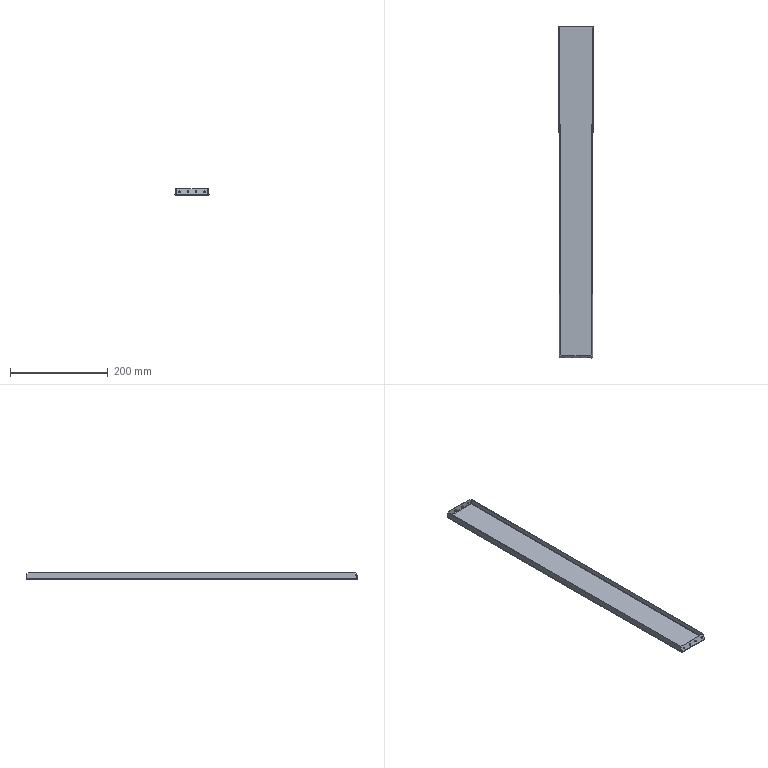Part | SolidWorks | features BaseBody 1 | 1 solid | 72 faces | box 70.086 x 678.331 x 12.79 mm | volume 32032 mm3 | plane 31 | cylinder 24 | spline 17 | commonest cylinder face diameters 3.2 x8 1.5 x6 2.5 x6 2 x4